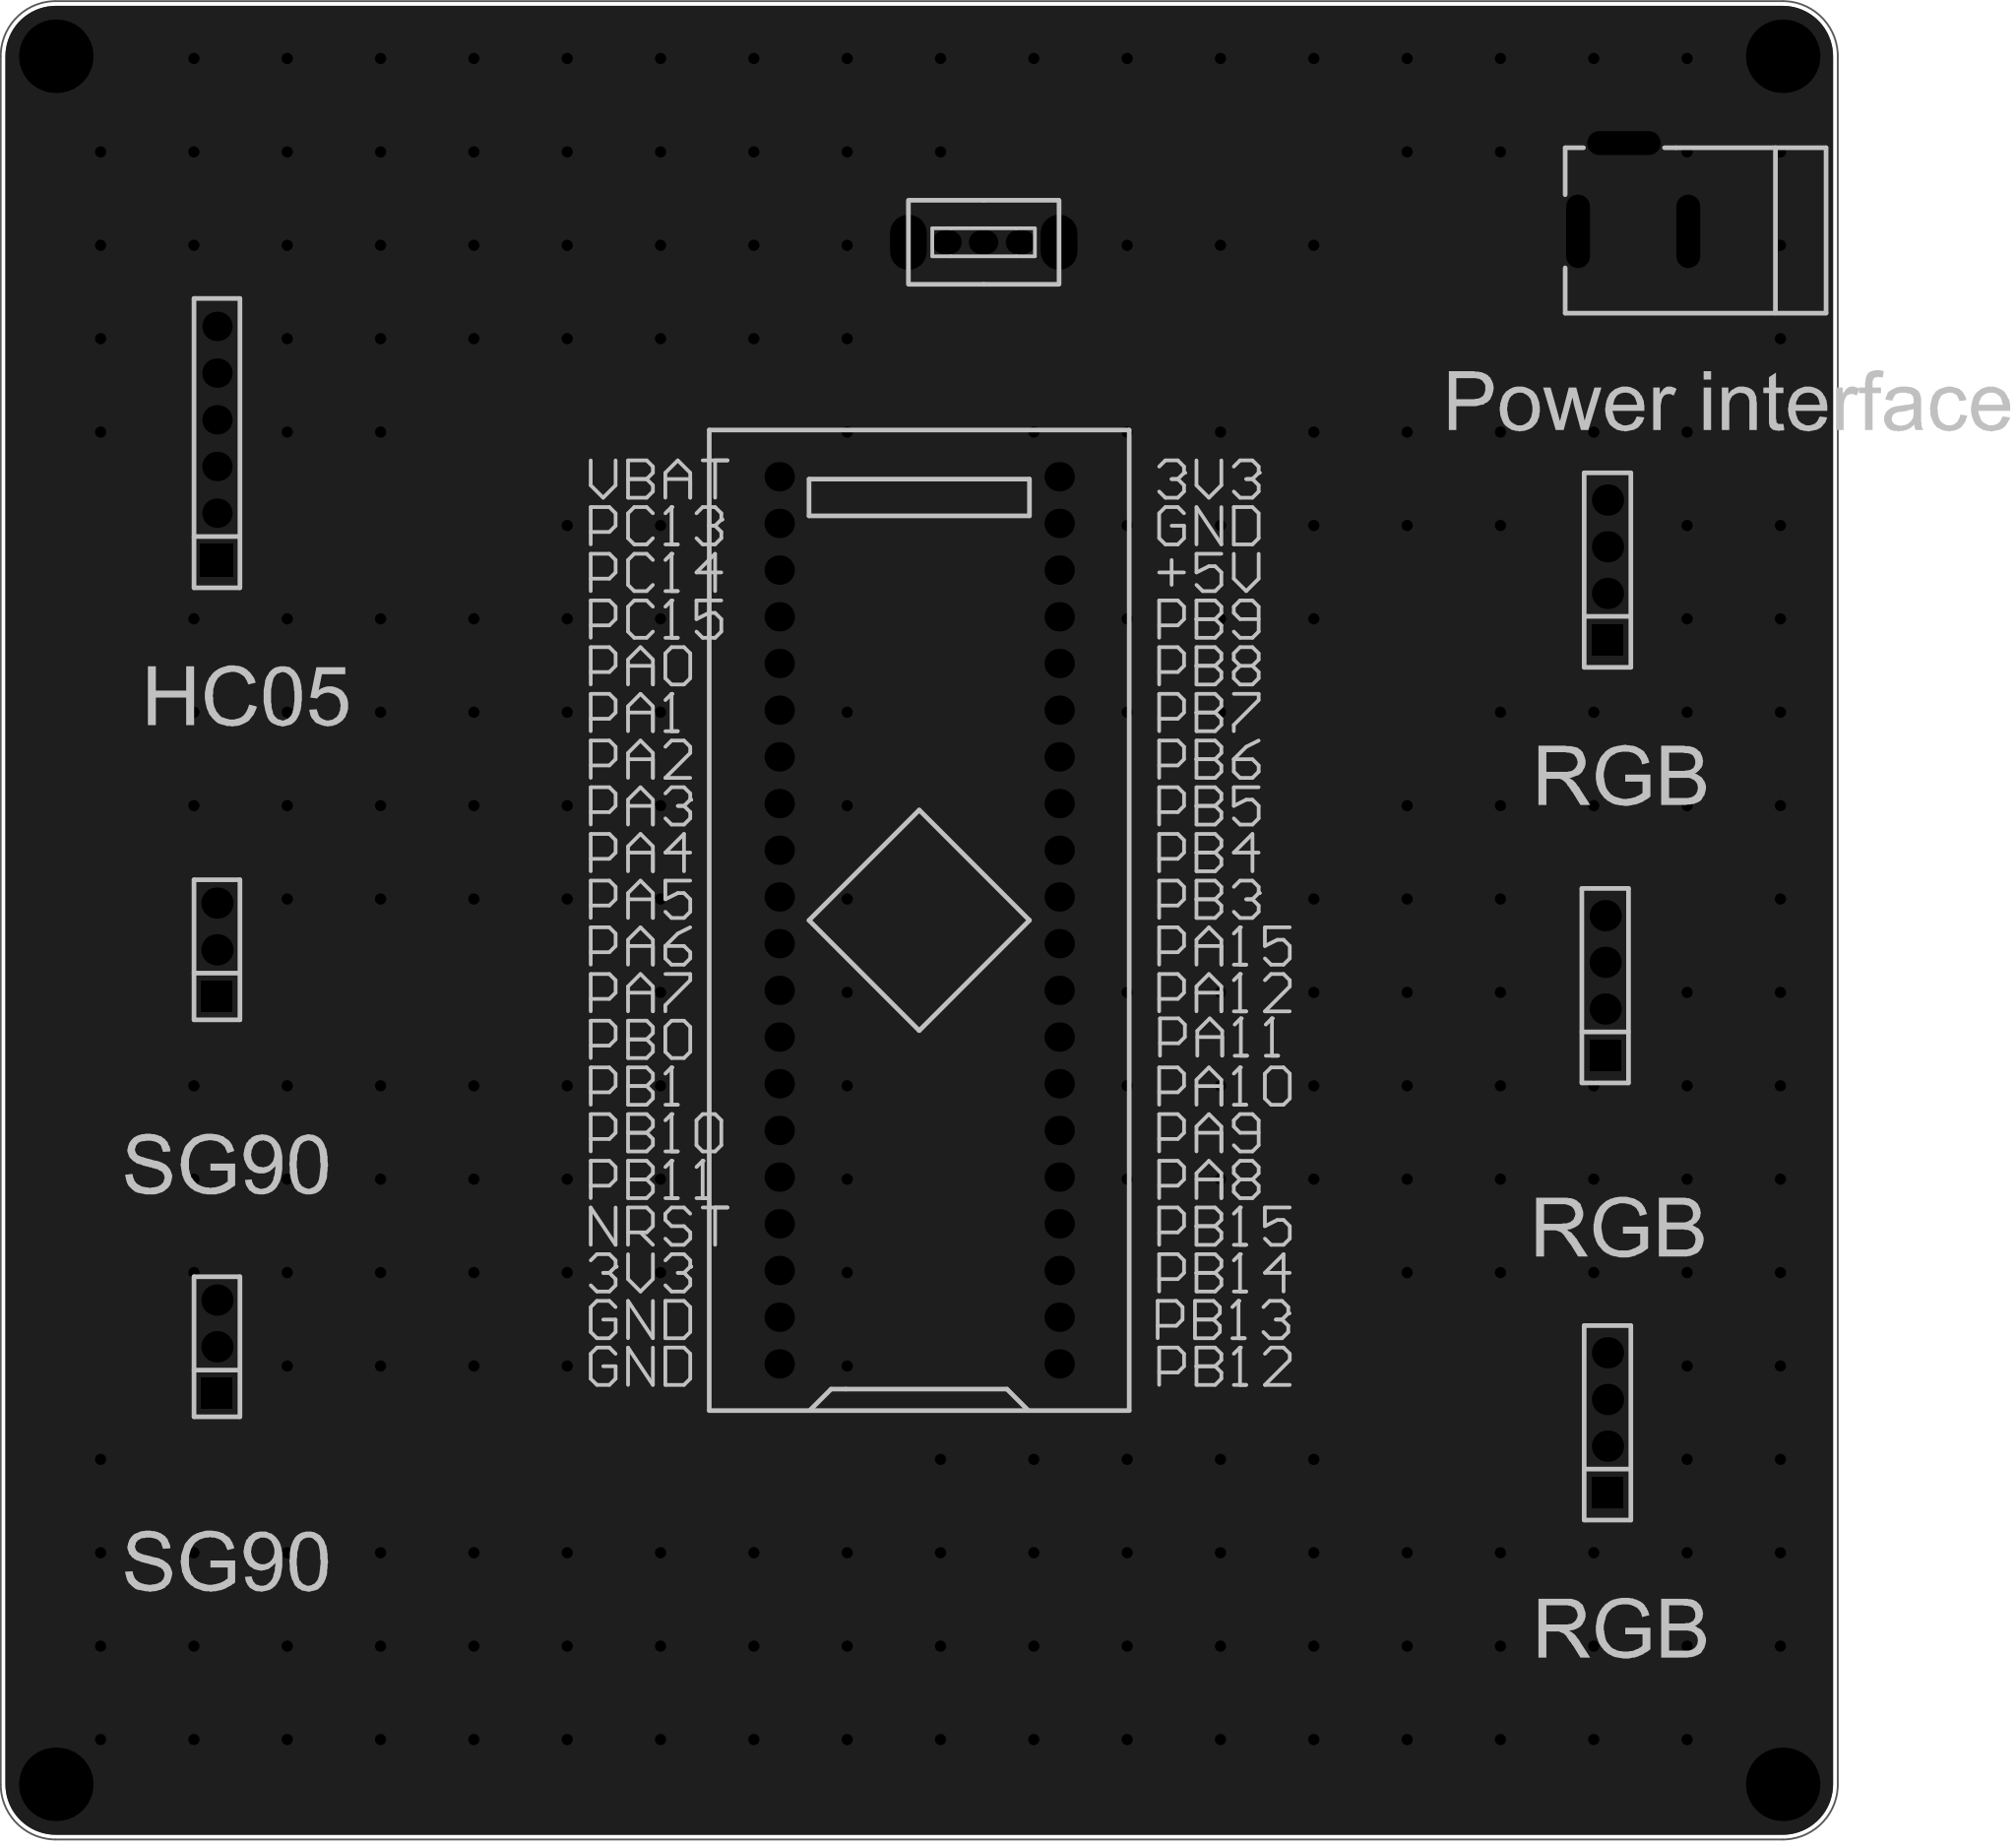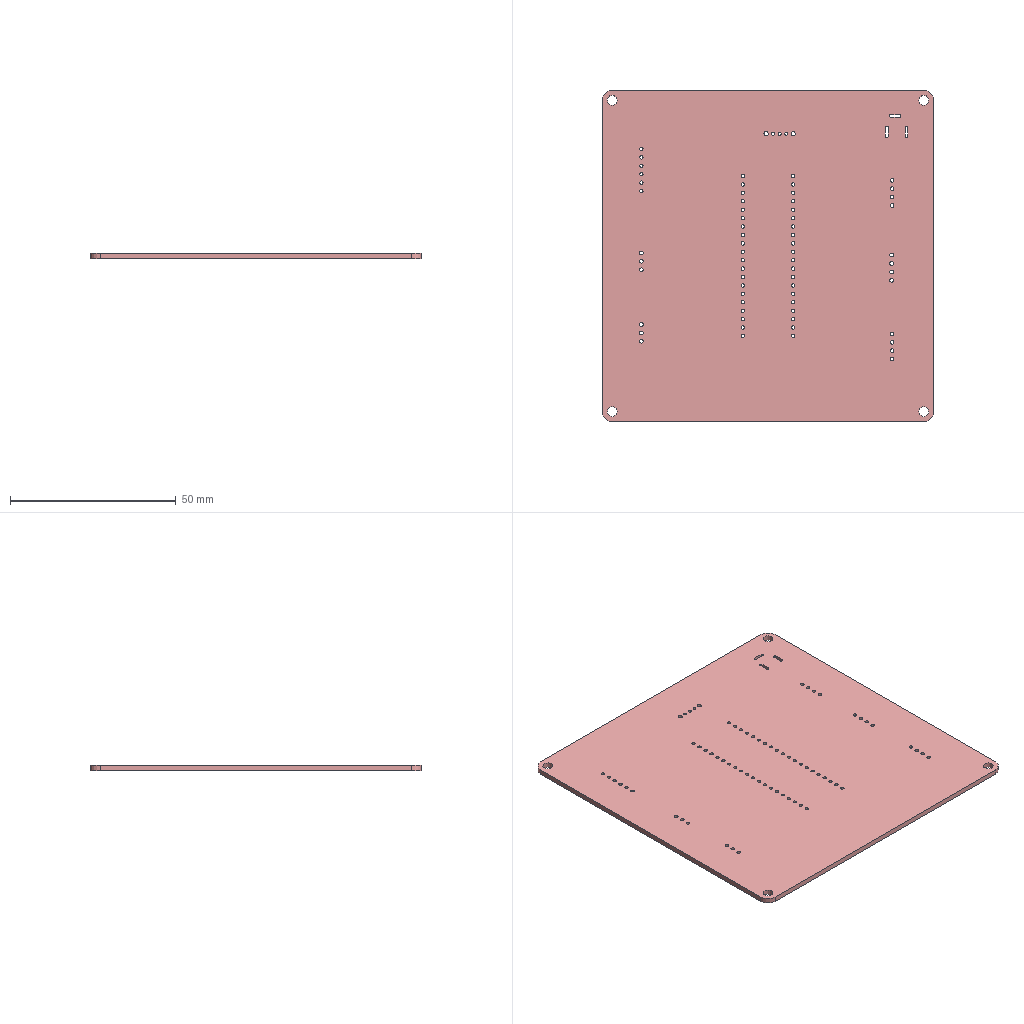Circuit board layout | Altium Designer | box 100 x 100 x 1.6 mm
Layer stack:
# Altium Designer layer stack of  (unit mm; dielectric type: 0 none, 1 core, 2 prepreg, 3 surface material)
index,name,kind,layer,copper_thickness_mm,dielectric_type,dielectric_thickness_mm,dielectric_material,dielectric_constant
0,Top Paste Mask Layer,other,,,,,,
1,Top Silkscreen Layer,other,,,,,,
2,Top Solder Mask Layer,dielectric,,,3,0.01,,3.3
3,Top Layer,copper,Top Layer,0.035,,,,
4,Dielectric1,dielectric,,,3,1.51,FR4,4.5
5,Bottom Layer,copper,Bottom Layer,0.035,,,,
6,Bottom Solder Mask Layer,dielectric,,,3,0.01,,3.3
7,Bottom Silkscreen Layer,other,,,,,,
8,Bottom Paste Mask Layer,other,,,,,,
# drill layer pairs: low layer,high layer
drill_pair,Top Layer,Bottom Layer
Part placement:
Designator,Comment,Layer,Footprint,Center-X(mm),Center-Y(mm),Rotation
U1,STM32F103C8T6-Card,TopLayer,CONN-TH_L53.3-W22.9_STM32F103C8T6-CARD,141.351,130.937,90
SW5,,TopLayer,拨动开关,144.861,167.819,0
DC1,,TopLayer,DC-2.0,180.213,170.815,0
H1,,TopLayer,HDR-TH_4P-P2.54-V-F,178.689,127.381,90
H2,,TopLayer,HDR-TH_4P-P2.54-V-F,178.816,103.602,90
H3,,TopLayer,HDR-TH_4P-P2.54-V-F,178.816,149.987,90
H4,,TopLayer,HDR-TH_3P-P2.54-V-M,103.124,129.334,90
H5,,TopLayer,HDR-TH_3P-P2.54-V-M,103.124,107.74,90
H6,,TopLayer,HDR-TH_6P-P2.54-V-F,103.124,156.893,90
Pad and via stacks:
# Altium Designer via and pad stacks of  (unit mm). Each distinct definition once, with the count of objects using it.
# via: kind,start_layer,end_layer,hole_mm,diameter_mm,mode(0 simple;1 top-mid-bottom;2 full stack),diameter_per_layer,count,example_net
# pad: kind,layer,hole_mm,hole_type(0 round;1 square;2 slot),plating,top_size,top_shape(1 round;2 rect;3 octagon;9 rounded rect),mid_size,bottom_size,mode,footprint,size_per_layer,count,example
pad,Multi-Layer,3,0,plated,4x4,1,4x4,4x4,0,,,4,1
pad,Multi-Layer,1,0,plated,1.6x1.6,1,1.6x1.6,1.6x1.6,0,CONN-TH_L53.3-W22.9_STM32F103C8T6-CARD,,40,U1.1
pad,Multi-Layer,0.8992,0,plated,1.6x1.3,1,1.6x1.3,1.6x1.3,0,\u00B2\u00A6\u00B6\u00AF\u00BF\u00AA\u00B9\u00D8,,3,SW5.1
pad,Multi-Layer,1.3,0,plated,3x1.999,1,3x1.999,3x1.999,0,\u00B2\u00A6\u00B6\u00AF\u00BF\u00AA\u00B9\u00D8,,2,SW5.4
pad,Multi-Layer,0.8001,2,plated,4x1.3,1,4x1.3,4x1.3,0,DC-2.0,,3,DC1.2
pad,Multi-Layer,1.1,0,plated,1.7x1.7,2,1.7x1.7,1.7x1.7,0,HDR-TH_4P-P2.54-V-F,,3,H1.1
pad,Multi-Layer,1.1,0,plated,1.7x1.7,1,1.7x1.7,1.7x1.7,0,HDR-TH_4P-P2.54-V-F,,9,H1.2
pad,Multi-Layer,1.1,0,plated,1.7x1.7,2,1.7x1.7,1.7x1.7,0,HDR-TH_3P-P2.54-V-M,,2,H4.1
pad,Multi-Layer,1.1,0,plated,1.7x1.7,1,1.7x1.7,1.7x1.7,0,HDR-TH_3P-P2.54-V-M,,4,H4.2
pad,Multi-Layer,1.02,0,plated,1.6x1.6,1,1.6x1.6,1.6x1.6,0,HDR-TH_6P-P2.54-V-F,,5,H6.6
pad,Multi-Layer,1.02,0,plated,1.8x1.8,2,1.8x1.8,1.8x1.8,0,HDR-TH_6P-P2.54-V-F,,1,H6.1
via,Top Layer,Bottom Layer,0.3048,0.61,0,,242,GND
Copper pours:
name,layer,net,type(0 solid;1 hatched;2 none)
Bottom Layer-GND,Bottom Layer,GND,0
Top Layer-GND,Top Layer,GND,0